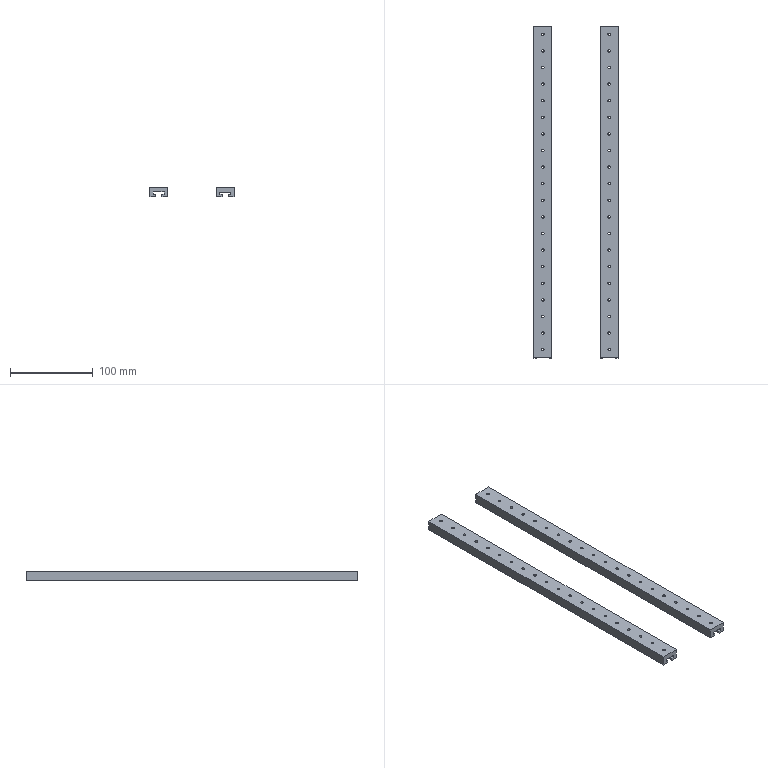Part | SolidWorks | 2 solids | 316 faces | box 102 x 400 x 12 mm | volume 159088 mm3 | cylinder 160 | cone 80 | plane 76 | commonest cylinder face diameters 3.1 x80 5.7 x80